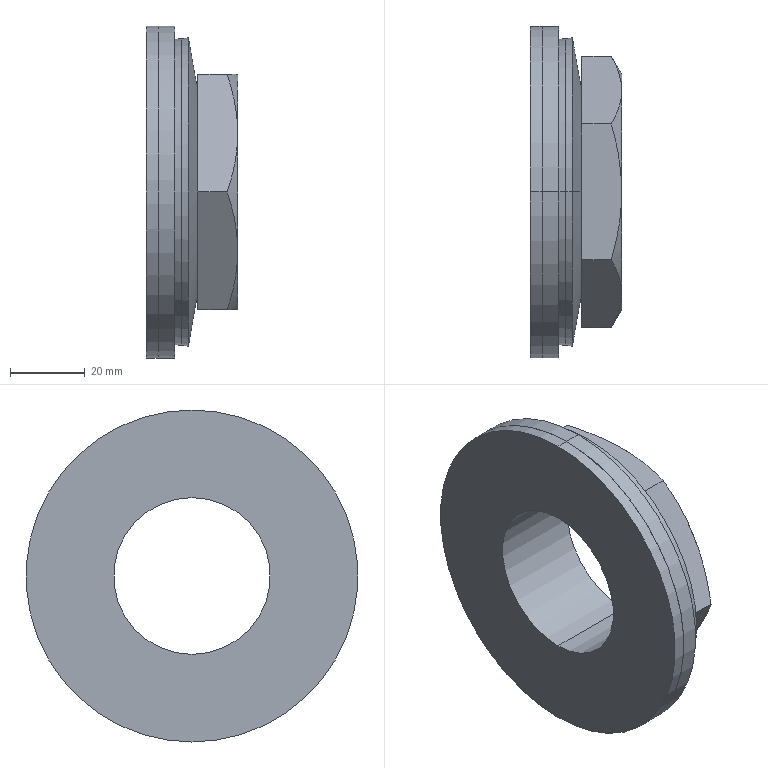Part | STEP file | TL350_2Parts | 1 solid | 34 faces | box 24.53 x 89 x 89 mm | volume 78902 mm3 | cone 14 | plane 12 | cylinder 8 | commonest cylinder face diameters 89 x4 42 x2 88 x2